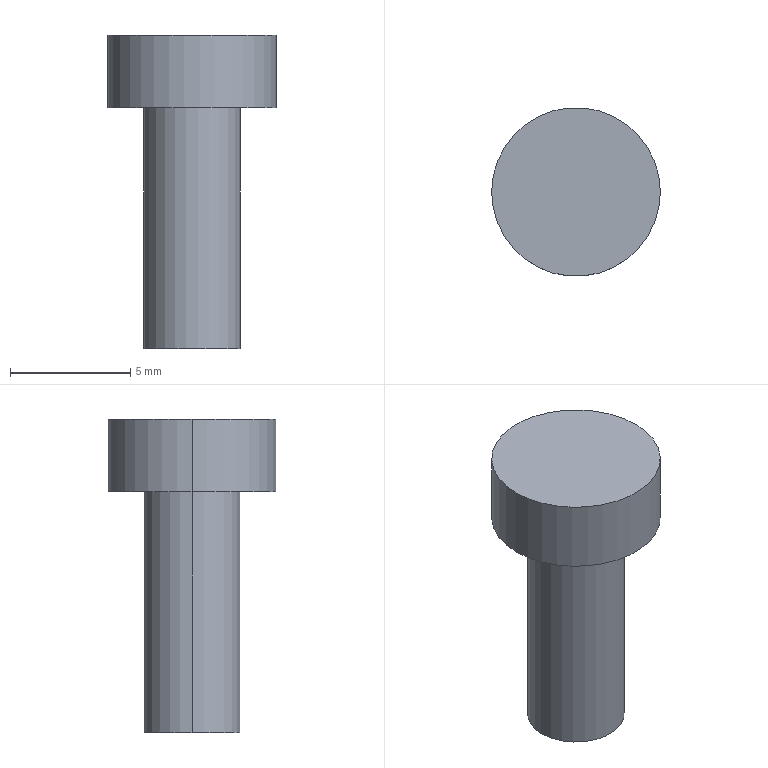Part | SolidWorks | features Extrusion 1, ICE 1 | 1 solid | 7 faces | box 7 x 7 x 13 mm | volume 241.117 mm3 | cylinder 4 | plane 3 | commonest cylinder face diameters 4 x2 7 x2
STEP:
#1=CARTESIAN_POINT('',(3.5,0.,3.));
#2=VERTEX_POINT('',#1);
#3=CARTESIAN_POINT('',(-3.5,0.,3.));
#4=VERTEX_POINT('',#3);
#5=CARTESIAN_POINT('',(0.,0.,3.));
#6=DIRECTION('',(0.,0.,1.));
#7=DIRECTION('',(1.,0.,0.));
#8=AXIS2_PLACEMENT_3D('',#5,#6,#7);
#9=CIRCLE('',#8,3.5);
#10=EDGE_CURVE('',#2,#4,#9,.T.);
#11=ORIENTED_EDGE('',*,*,#10,.F.);
#12=CARTESIAN_POINT('',(3.5,0.,0.));
#13=VERTEX_POINT('',#12);
#14=CARTESIAN_POINT('',(3.5,0.,3.));
#15=DIRECTION('',(0.,0.,-1.));
#16=VECTOR('',#15,1000.);
#17=LINE('',#14,#16);
#18=EDGE_CURVE('',#2,#13,#17,.T.);
#19=ORIENTED_EDGE('',*,*,#18,.T.);
#20=CARTESIAN_POINT('',(-3.5,0.,0.));
#21=VERTEX_POINT('',#20);
#22=CARTESIAN_POINT('',(0.,0.,0.));
#23=DIRECTION('',(0.,0.,1.));
#24=DIRECTION('',(1.,0.,0.));
#25=AXIS2_PLACEMENT_3D('',#22,#23,#24);
#26=CIRCLE('',#25,3.5);
#27=EDGE_CURVE('',#13,#21,#26,.T.);
#28=ORIENTED_EDGE('',*,*,#27,.T.);
#29=CARTESIAN_POINT('',(-3.5,0.,3.));
#30=DIRECTION('',(0.,0.,-1.));
#31=VECTOR('',#30,1000.);
#32=LINE('',#29,#31);
#33=EDGE_CURVE('',#4,#21,#32,.T.);
#34=ORIENTED_EDGE('',*,*,#33,.F.);
#35=EDGE_LOOP('',(#11,#19,#28,#34));
#36=FACE_OUTER_BOUND('',#35,.T.);
#37=CARTESIAN_POINT('',(0.,0.,3.));
#38=DIRECTION('',(0.,0.,-1.));
#39=DIRECTION('',(-1.,0.,0.));
#40=AXIS2_PLACEMENT_3D('',#37,#38,#39);
#41=CYLINDRICAL_SURFACE('',#40,3.5);
#42=ADVANCED_FACE('',(#36),#41,.T.);
#43=CARTESIAN_POINT('',(2.,0.,-10.));
#44=VERTEX_POINT('',#43);
#45=CARTESIAN_POINT('',(-2.,0.,-10.));
#46=VERTEX_POINT('',#45);
#47=CARTESIAN_POINT('',(0.,0.,-10.));
#48=DIRECTION('',(0.,0.,1.));
#49=DIRECTION('',(1.,0.,0.));
#50=AXIS2_PLACEMENT_3D('',#47,#48,#49);
#51=CIRCLE('',#50,2.);
#52=EDGE_CURVE('',#44,#46,#51,.T.);
#53=ORIENTED_EDGE('',*,*,#52,.T.);
#54=CARTESIAN_POINT('',(-2.,0.,0.));
#55=VERTEX_POINT('',#54);
#56=CARTESIAN_POINT('',(-2.,0.,-10.));
#57=DIRECTION('',(0.,0.,1.));
#58=VECTOR('',#57,1000.);
#59=LINE('',#56,#58);
#60=EDGE_CURVE('',#46,#55,#59,.T.);
#61=ORIENTED_EDGE('',*,*,#60,.T.);
#62=CARTESIAN_POINT('',(2.,0.,0.));
#63=VERTEX_POINT('',#62);
#64=CARTESIAN_POINT('',(0.,0.,0.));
#65=DIRECTION('',(0.,0.,1.));
#66=DIRECTION('',(1.,0.,0.));
#67=AXIS2_PLACEMENT_3D('',#64,#65,#66);
#68=CIRCLE('',#67,2.);
#69=EDGE_CURVE('',#63,#55,#68,.T.);
#70=ORIENTED_EDGE('',*,*,#69,.F.);
#71=CARTESIAN_POINT('',(2.,0.,-10.));
#72=DIRECTION('',(0.,0.,1.));
#73=VECTOR('',#72,1000.);
#74=LINE('',#71,#73);
#75=EDGE_CURVE('',#44,#63,#74,.T.);
#76=ORIENTED_EDGE('',*,*,#75,.F.);
#77=EDGE_LOOP('',(#53,#61,#70,#76));
#78=FACE_OUTER_BOUND('',#77,.T.);
#79=CARTESIAN_POINT('',(0.,0.,-10.));
#80=DIRECTION('',(0.,0.,1.));
#81=DIRECTION('',(1.,0.,0.));
#82=AXIS2_PLACEMENT_3D('',#79,#80,#81);
#83=CYLINDRICAL_SURFACE('',#82,2.);
#84=ADVANCED_FACE('',(#78),#83,.T.);
#85=ORIENTED_EDGE('',*,*,#60,.F.);
#86=CARTESIAN_POINT('',(0.,0.,-10.));
#87=DIRECTION('',(0.,0.,1.));
#88=DIRECTION('',(1.,0.,0.));
#89=AXIS2_PLACEMENT_3D('',#86,#87,#88);
#90=CIRCLE('',#89,2.);
#91=EDGE_CURVE('',#46,#44,#90,.T.);
#92=ORIENTED_EDGE('',*,*,#91,.T.);
#93=ORIENTED_EDGE('',*,*,#75,.T.);
#94=CARTESIAN_POINT('',(0.,0.,0.));
#95=DIRECTION('',(0.,0.,1.));
#96=DIRECTION('',(1.,0.,0.));
#97=AXIS2_PLACEMENT_3D('',#94,#95,#96);
#98=CIRCLE('',#97,2.);
#99=EDGE_CURVE('',#55,#63,#98,.T.);
#100=ORIENTED_EDGE('',*,*,#99,.F.);
#101=EDGE_LOOP('',(#85,#92,#93,#100));
#102=FACE_OUTER_BOUND('',#101,.T.);
#103=CARTESIAN_POINT('',(0.,0.,-10.));
#104=DIRECTION('',(0.,0.,1.));
#105=DIRECTION('',(1.,0.,0.));
#106=AXIS2_PLACEMENT_3D('',#103,#104,#105);
#107=CYLINDRICAL_SURFACE('',#106,2.);
#108=ADVANCED_FACE('',(#102),#107,.T.);
#109=ORIENTED_EDGE('',*,*,#52,.F.);
#110=ORIENTED_EDGE('',*,*,#91,.F.);
#111=EDGE_LOOP('',(#109,#110));
#112=FACE_OUTER_BOUND('',#111,.T.);
#113=CARTESIAN_POINT('',(0.,0.,-10.));
#114=DIRECTION('',(0.,0.,1.));
#115=DIRECTION('',(1.,0.,0.));
#116=AXIS2_PLACEMENT_3D('',#113,#114,#115);
#117=PLANE('',#116);
#118=ADVANCED_FACE('',(#112),#117,.F.);
#119=ORIENTED_EDGE('',*,*,#18,.F.);
#120=CARTESIAN_POINT('',(0.,0.,3.));
#121=DIRECTION('',(0.,0.,1.));
#122=DIRECTION('',(1.,0.,0.));
#123=AXIS2_PLACEMENT_3D('',#120,#121,#122);
#124=CIRCLE('',#123,3.5);
#125=EDGE_CURVE('',#4,#2,#124,.T.);
#126=ORIENTED_EDGE('',*,*,#125,.F.);
#127=ORIENTED_EDGE('',*,*,#33,.T.);
#128=CARTESIAN_POINT('',(0.,0.,0.));
#129=DIRECTION('',(0.,0.,1.));
#130=DIRECTION('',(1.,0.,0.));
#131=AXIS2_PLACEMENT_3D('',#128,#129,#130);
#132=CIRCLE('',#131,3.5);
#133=EDGE_CURVE('',#21,#13,#132,.T.);
#134=ORIENTED_EDGE('',*,*,#133,.T.);
#135=EDGE_LOOP('',(#119,#126,#127,#134));
#136=FACE_OUTER_BOUND('',#135,.T.);
#137=CARTESIAN_POINT('',(0.,0.,3.));
#138=DIRECTION('',(0.,0.,-1.));
#139=DIRECTION('',(-1.,0.,0.));
#140=AXIS2_PLACEMENT_3D('',#137,#138,#139);
#141=CYLINDRICAL_SURFACE('',#140,3.5);
#142=ADVANCED_FACE('',(#136),#141,.T.);
#143=ORIENTED_EDGE('',*,*,#125,.T.);
#144=ORIENTED_EDGE('',*,*,#10,.T.);
#145=EDGE_LOOP('',(#143,#144));
#146=FACE_OUTER_BOUND('',#145,.T.);
#147=CARTESIAN_POINT('',(0.,0.,3.));
#148=DIRECTION('',(0.,0.,1.));
#149=DIRECTION('',(1.,0.,0.));
#150=AXIS2_PLACEMENT_3D('',#147,#148,#149);
#151=PLANE('',#150);
#152=ADVANCED_FACE('',(#146),#151,.T.);
#153=ORIENTED_EDGE('',*,*,#69,.T.);
#154=ORIENTED_EDGE('',*,*,#99,.T.);
#155=EDGE_LOOP('',(#153,#154));
#156=FACE_BOUND('',#155,.T.);
#157=ORIENTED_EDGE('',*,*,#133,.F.);
#158=ORIENTED_EDGE('',*,*,#27,.F.);
#159=EDGE_LOOP('',(#157,#158));
#160=FACE_OUTER_BOUND('',#159,.T.);
#161=CARTESIAN_POINT('',(0.,0.,0.));
#162=DIRECTION('',(0.,0.,1.));
#163=DIRECTION('',(1.,0.,0.));
#164=AXIS2_PLACEMENT_3D('',#161,#162,#163);
#165=PLANE('',#164);
#166=ADVANCED_FACE('',(#156,#160),#165,.F.);
#167=CLOSED_SHELL('',(#42,#84,#108,#118,#142,#152,#166));
#168=MANIFOLD_SOLID_BREP('',#167);
#169=CARTESIAN_POINT('',(0.,0.,0.));
#170=DIRECTION('',(0.,0.,1.));
#171=DIRECTION('',(1.,0.,0.));
#172=AXIS2_PLACEMENT_3D('',#169,#170,#171);
#173=(LENGTH_UNIT()NAMED_UNIT(*)SI_UNIT(.MILLI.,.METRE.));
#174=UNCERTAINTY_MEASURE_WITH_UNIT(LENGTH_MEASURE(0.00001),#173,'','');
#175=(NAMED_UNIT(*)PLANE_ANGLE_UNIT()SI_UNIT($,.RADIAN.));
#176=(NAMED_UNIT(*)SI_UNIT($,.STERADIAN.)SOLID_ANGLE_UNIT());
#177=(GEOMETRIC_REPRESENTATION_CONTEXT(3)GLOBAL_UNCERTAINTY_ASSIGNED_CONTEXT((#174))GLOBAL_UNIT_ASSIGNED_CONTEXT((#173,#175,#176))REPRESENTATION_CONTEXT('',''));
#178=ADVANCED_BREP_SHAPE_REPRESENTATION('',(#168,#172),#177);